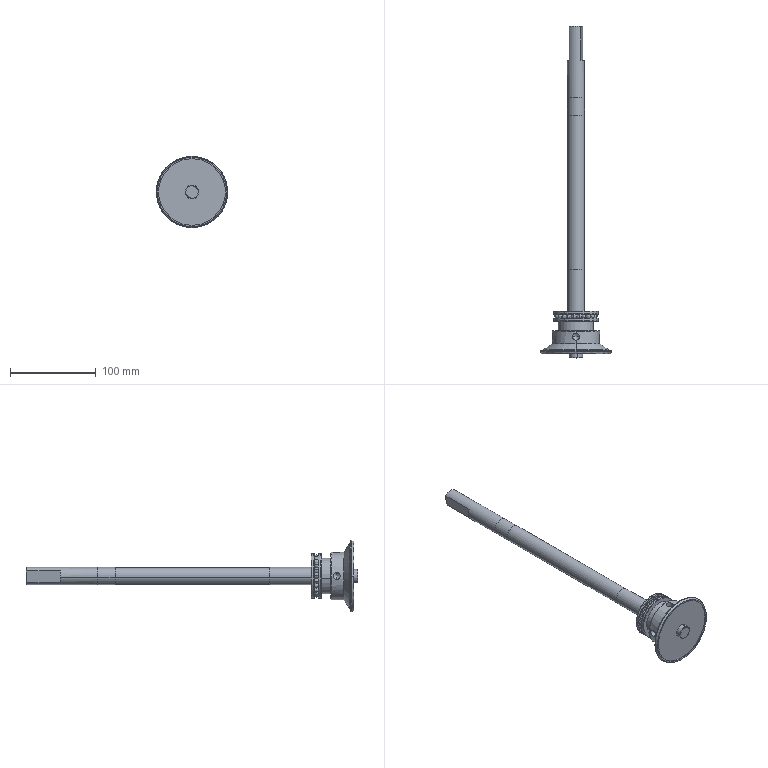Part | SolidWorks | 6 solids | 213 faces | box 83.227 x 387.8 x 83.227 mm | volume 211177 mm3 | spline 106 | cylinder 50 | plane 33 | cone 24 | commonest cylinder face diameters 20 x6 25 x6 8 x4 35 x4 52 x4 12 x2